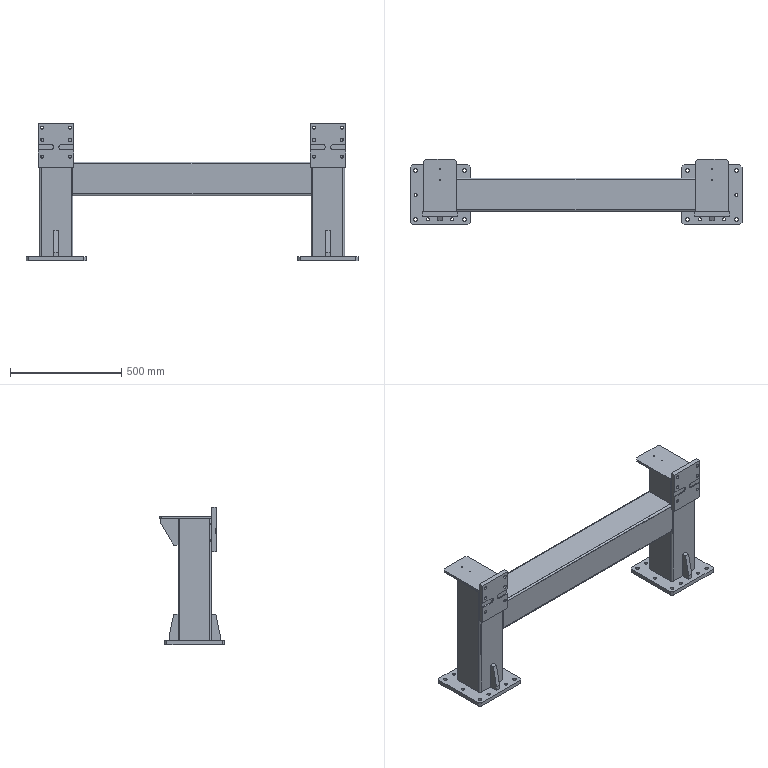Part | SolidWorks | features ICE 6, HoleWzd 5, Chamfer 4, 3DProfileFeature 1, MirrorPattern 1, WeldMemberFeat 1, WeldmentFeature 1 | 10 solids | 255 faces | box 1490 x 295 x 618 mm | volume 10128705 mm3 | plane 131 | cylinder 120 | cone 4 | commonest cylinder face diameters 14 x64 16.5 x16 8 x12 16 x12 5 x10 25 x6